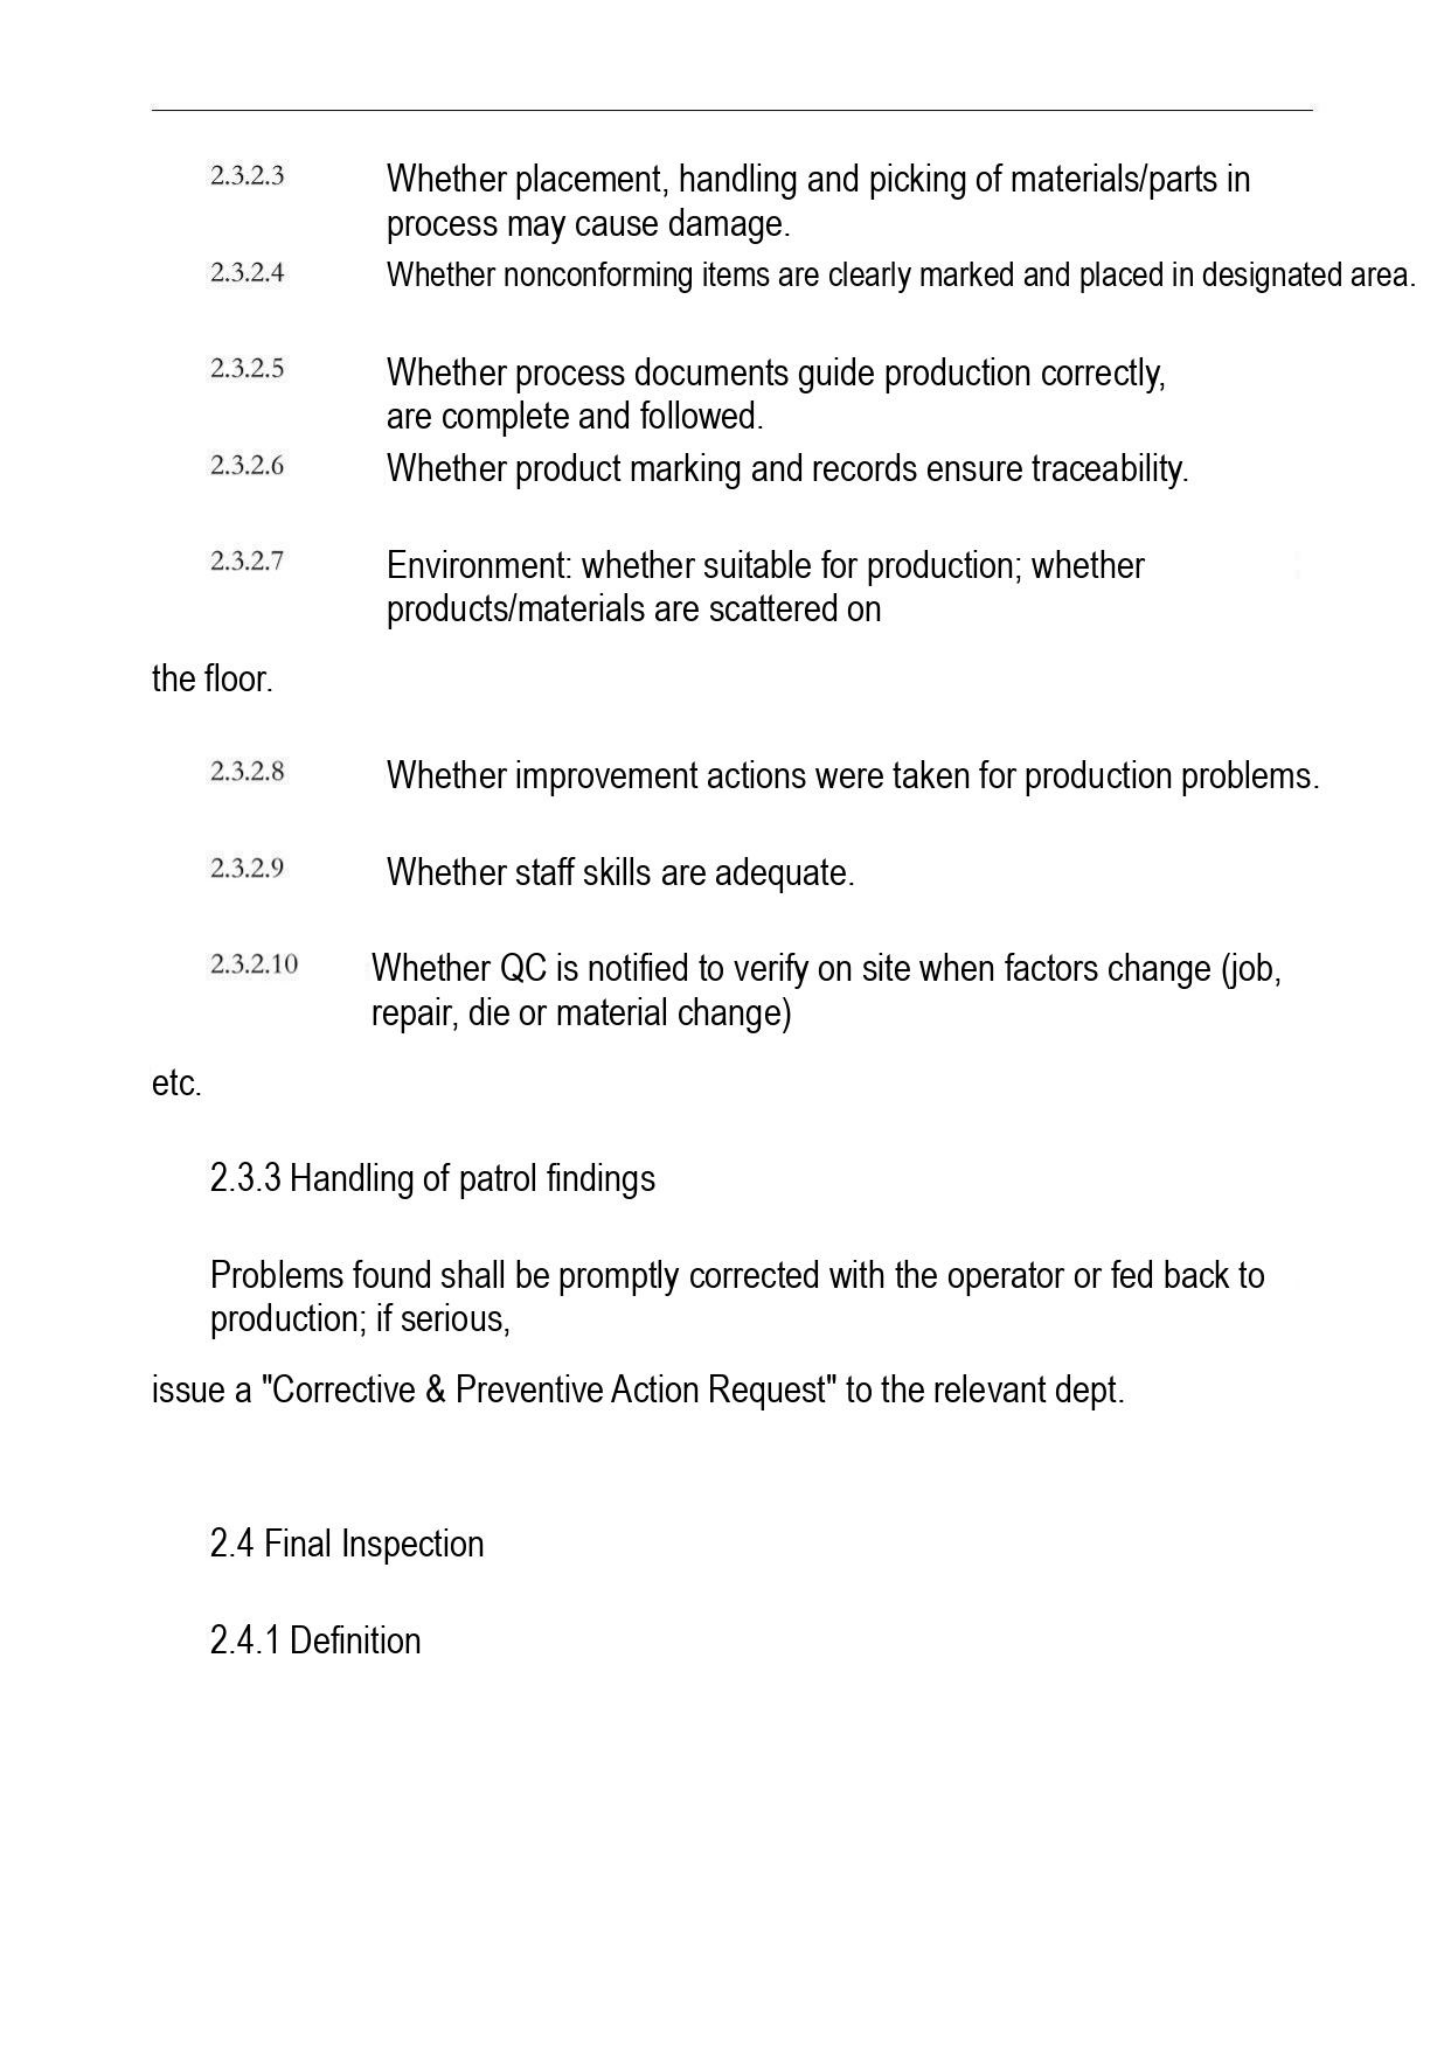2.3.2.3 Whether placement, handling and picking of materials/parts in process may cause damage.

2.3.2.4 Whether nonconforming items are clearly marked and placed in designated area.

2.3.2.5 Whether process documents guide production correctly, are complete and followed.

2.3.2.6 Whether product marking and records ensure traceability.

2.3.2.7 Environment: whether suitable for production; whether products/materials are scattered on

the floor.

2.3.2.8 Whether improvement actions were taken for production problems.

2.3.2.9 Whether staff skills are adequate.

2.3.2.10 Whether QC is notified to verify on site when factors change (job, repair, die or material change)

etc.

2.3.3 Handling of patrol findings

Problems found shall be promptly corrected with the operator or fed back to production; if serious,

issue a "Corrective & Preventive Action Request" to the relevant dept.

2.4 Final Inspection

2.4.1 Definition
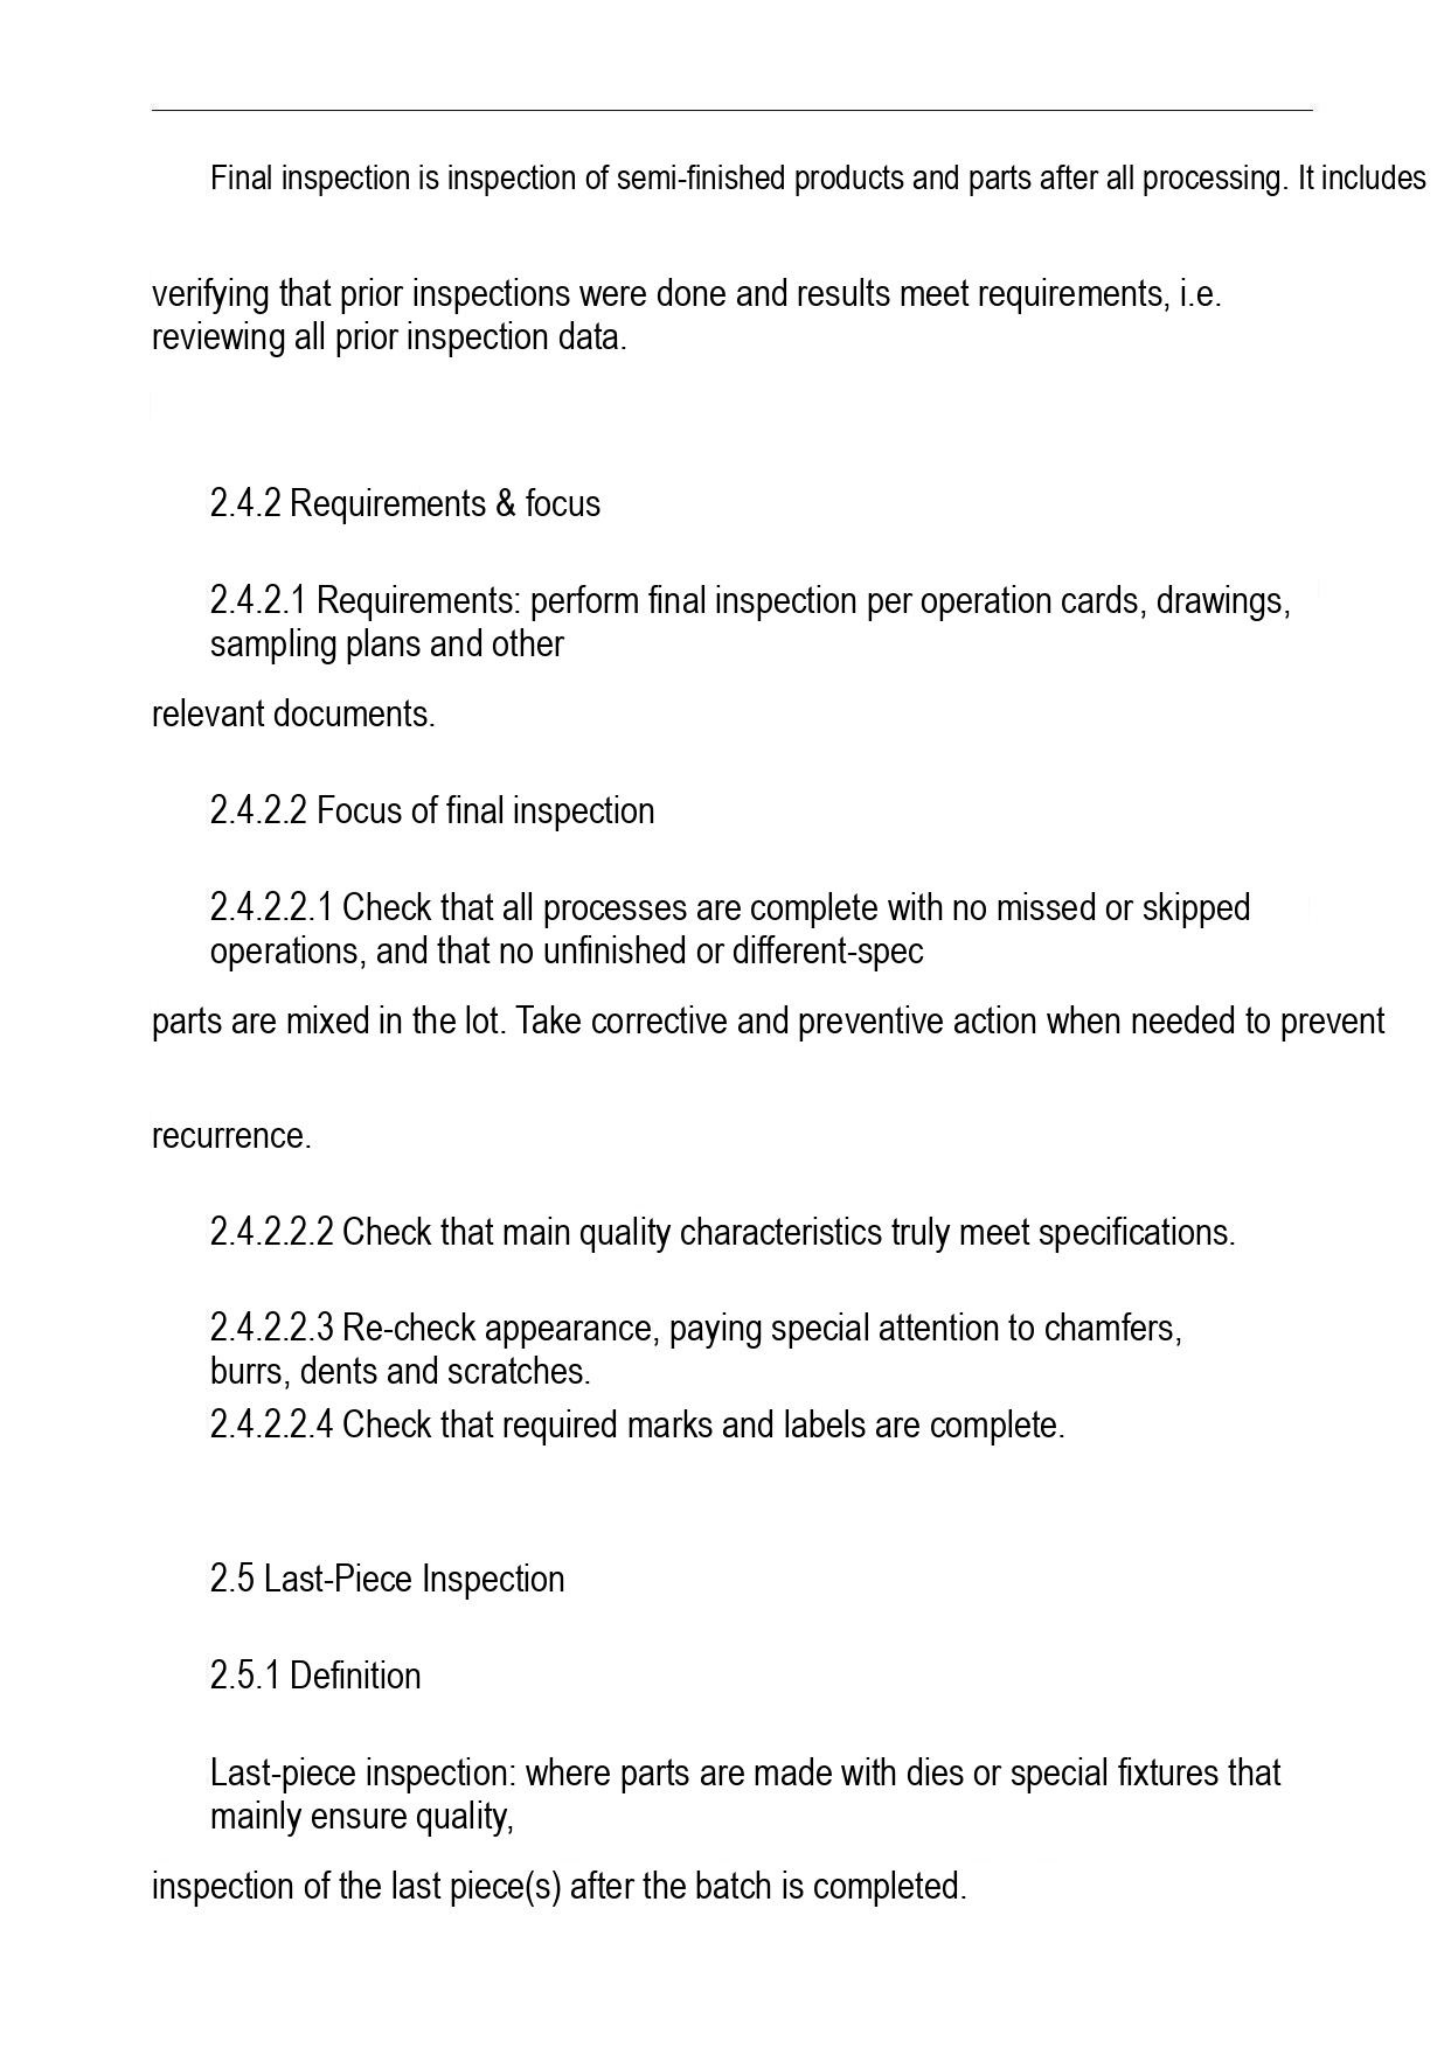Final inspection is inspection of semi-finished products and parts after all processing. It includes verifying that prior inspections were done and results meet requirements, i.e. reviewing all prior inspection data.

2.4.2 Requirements & focus

2.4.2.1 Requirements: perform final inspection per operation cards, drawings, sampling plans and other relevant documents.

2.4.2.2 Focus of final inspection

2.4.2.2.1 Check that all processes are complete with no missed or skipped operations, and that no unfinished or different-spec parts are mixed in the lot. Take corrective and preventive action when needed to prevent recurrence.

2.4.2.2.2 Check that main quality characteristics truly meet specifications.

2.4.2.2.3 Re-check appearance, paying special attention to chamfers, burrs, dents and scratches.

2.4.2.2.4 Check that required marks and labels are complete.

2.5 Last-Piece Inspection

2.5.1 Definition

Last-piece inspection: where parts are made with dies or special fixtures that mainly ensure quality, inspection of the last piece(s) after the batch is completed.
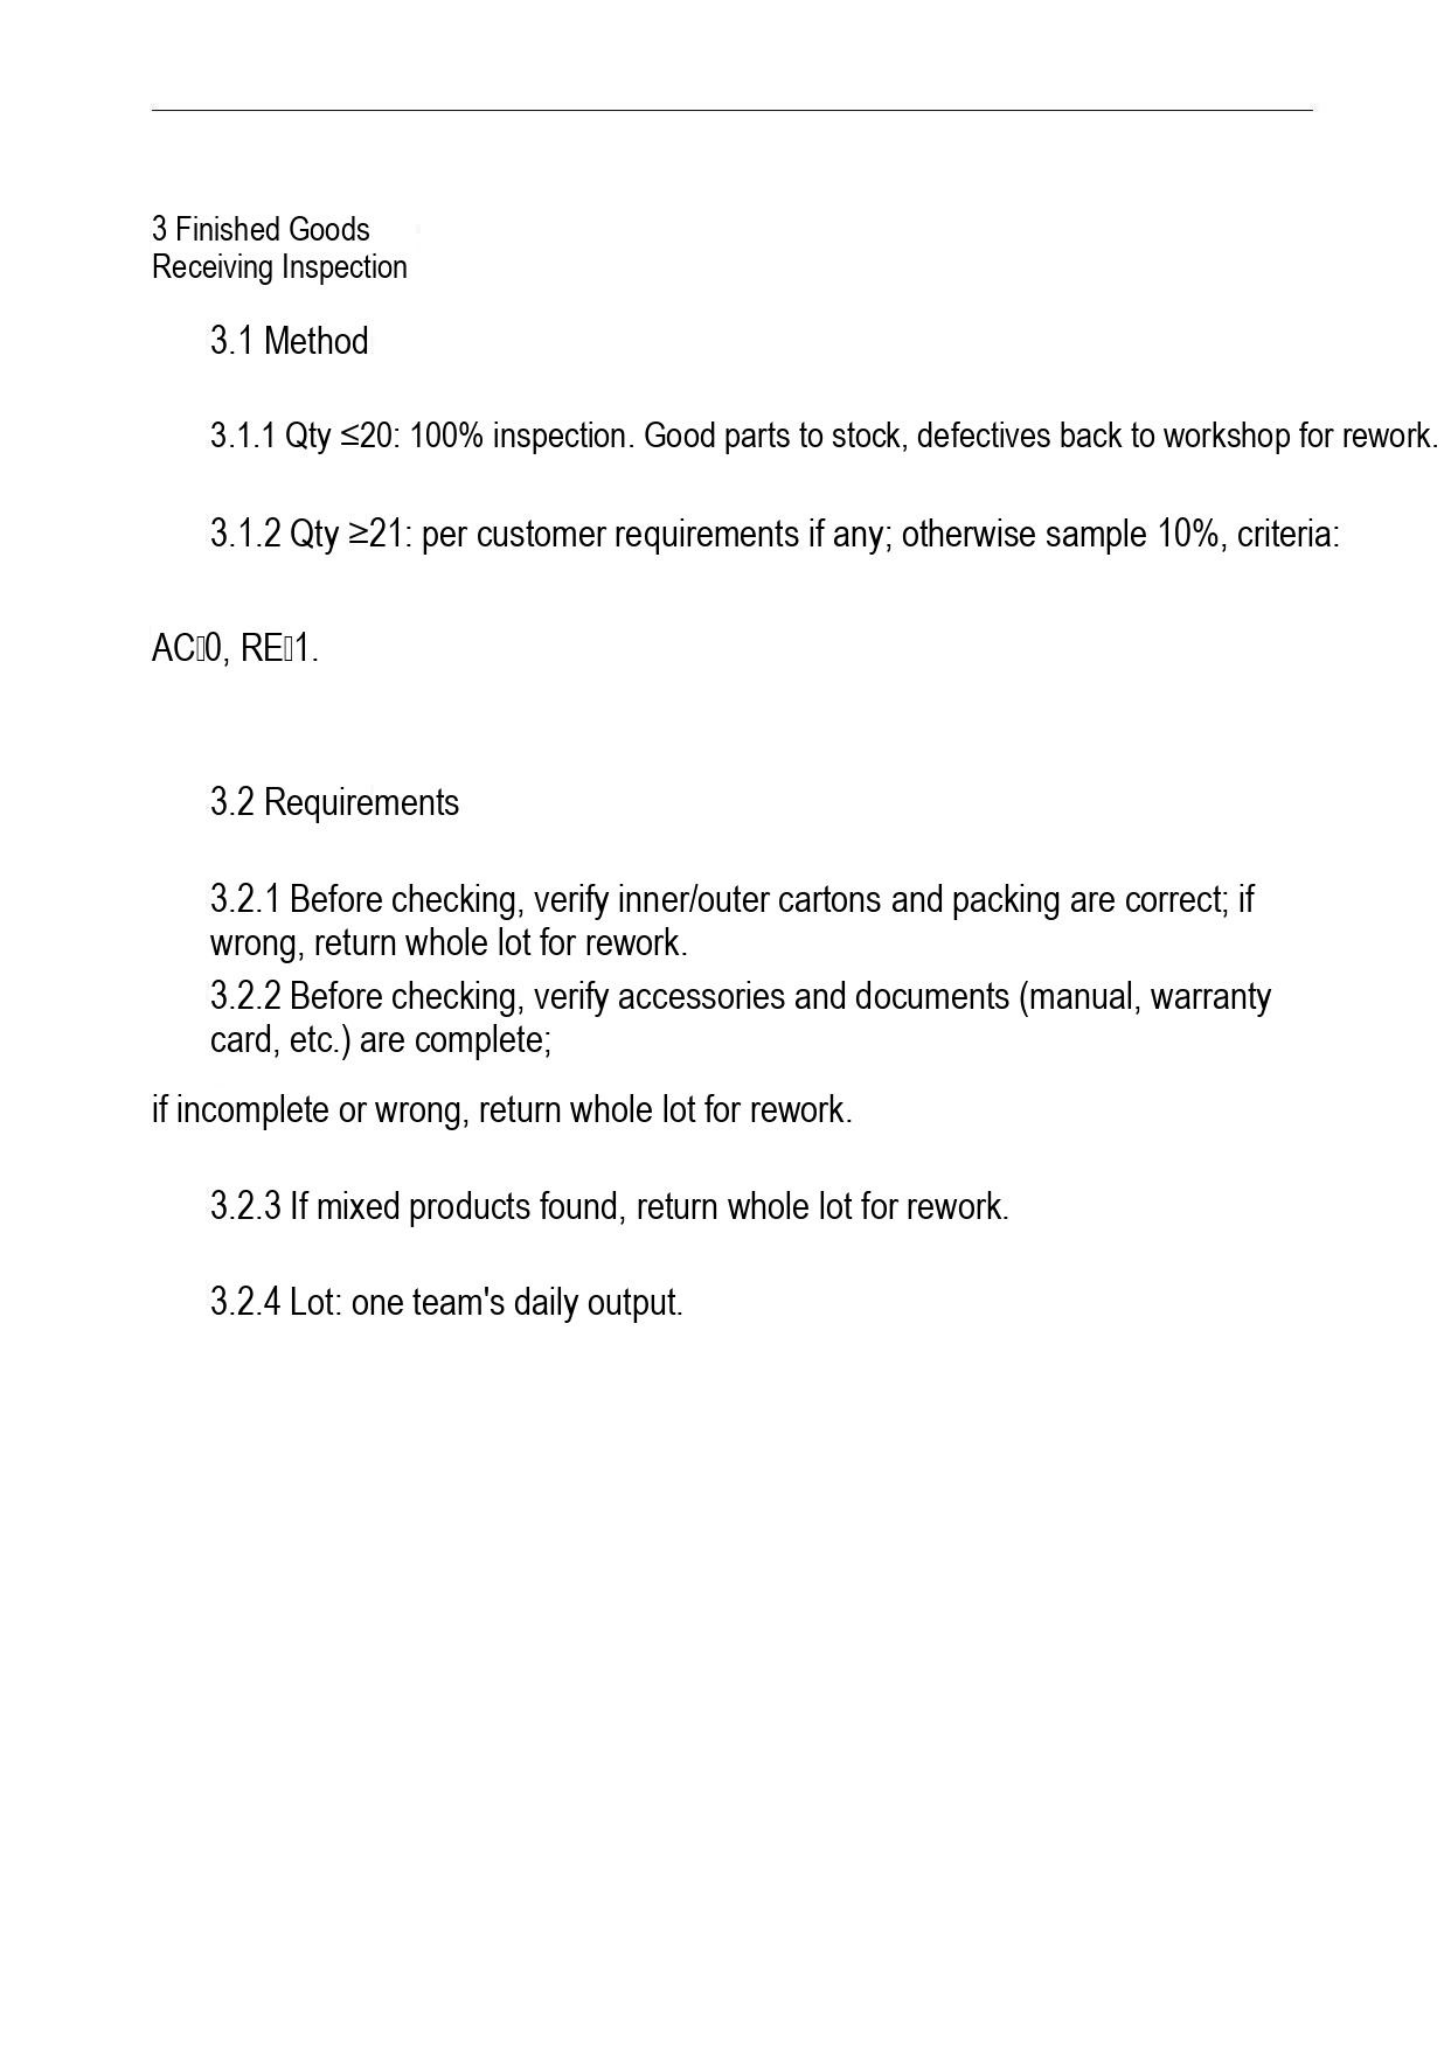3 Finished Goods
Receiving Inspection

3.1 Method

3.1.1 Qty ≤20: 100% inspection. Good parts to stock, defectives back to workshop for rework.

3.1.2 Qty ≥21: per customer requirements if any; otherwise sample 10%, criteria:

AC0, RE1.

3.2 Requirements

3.2.1 Before checking, verify inner/outer cartons and packing are correct; if wrong, return whole lot for rework.

3.2.2 Before checking, verify accessories and documents (manual, warranty card, etc.) are complete;

if incomplete or wrong, return whole lot for rework.

3.2.3 If mixed products found, return whole lot for rework.

3.2.4 Lot: one team's daily output.
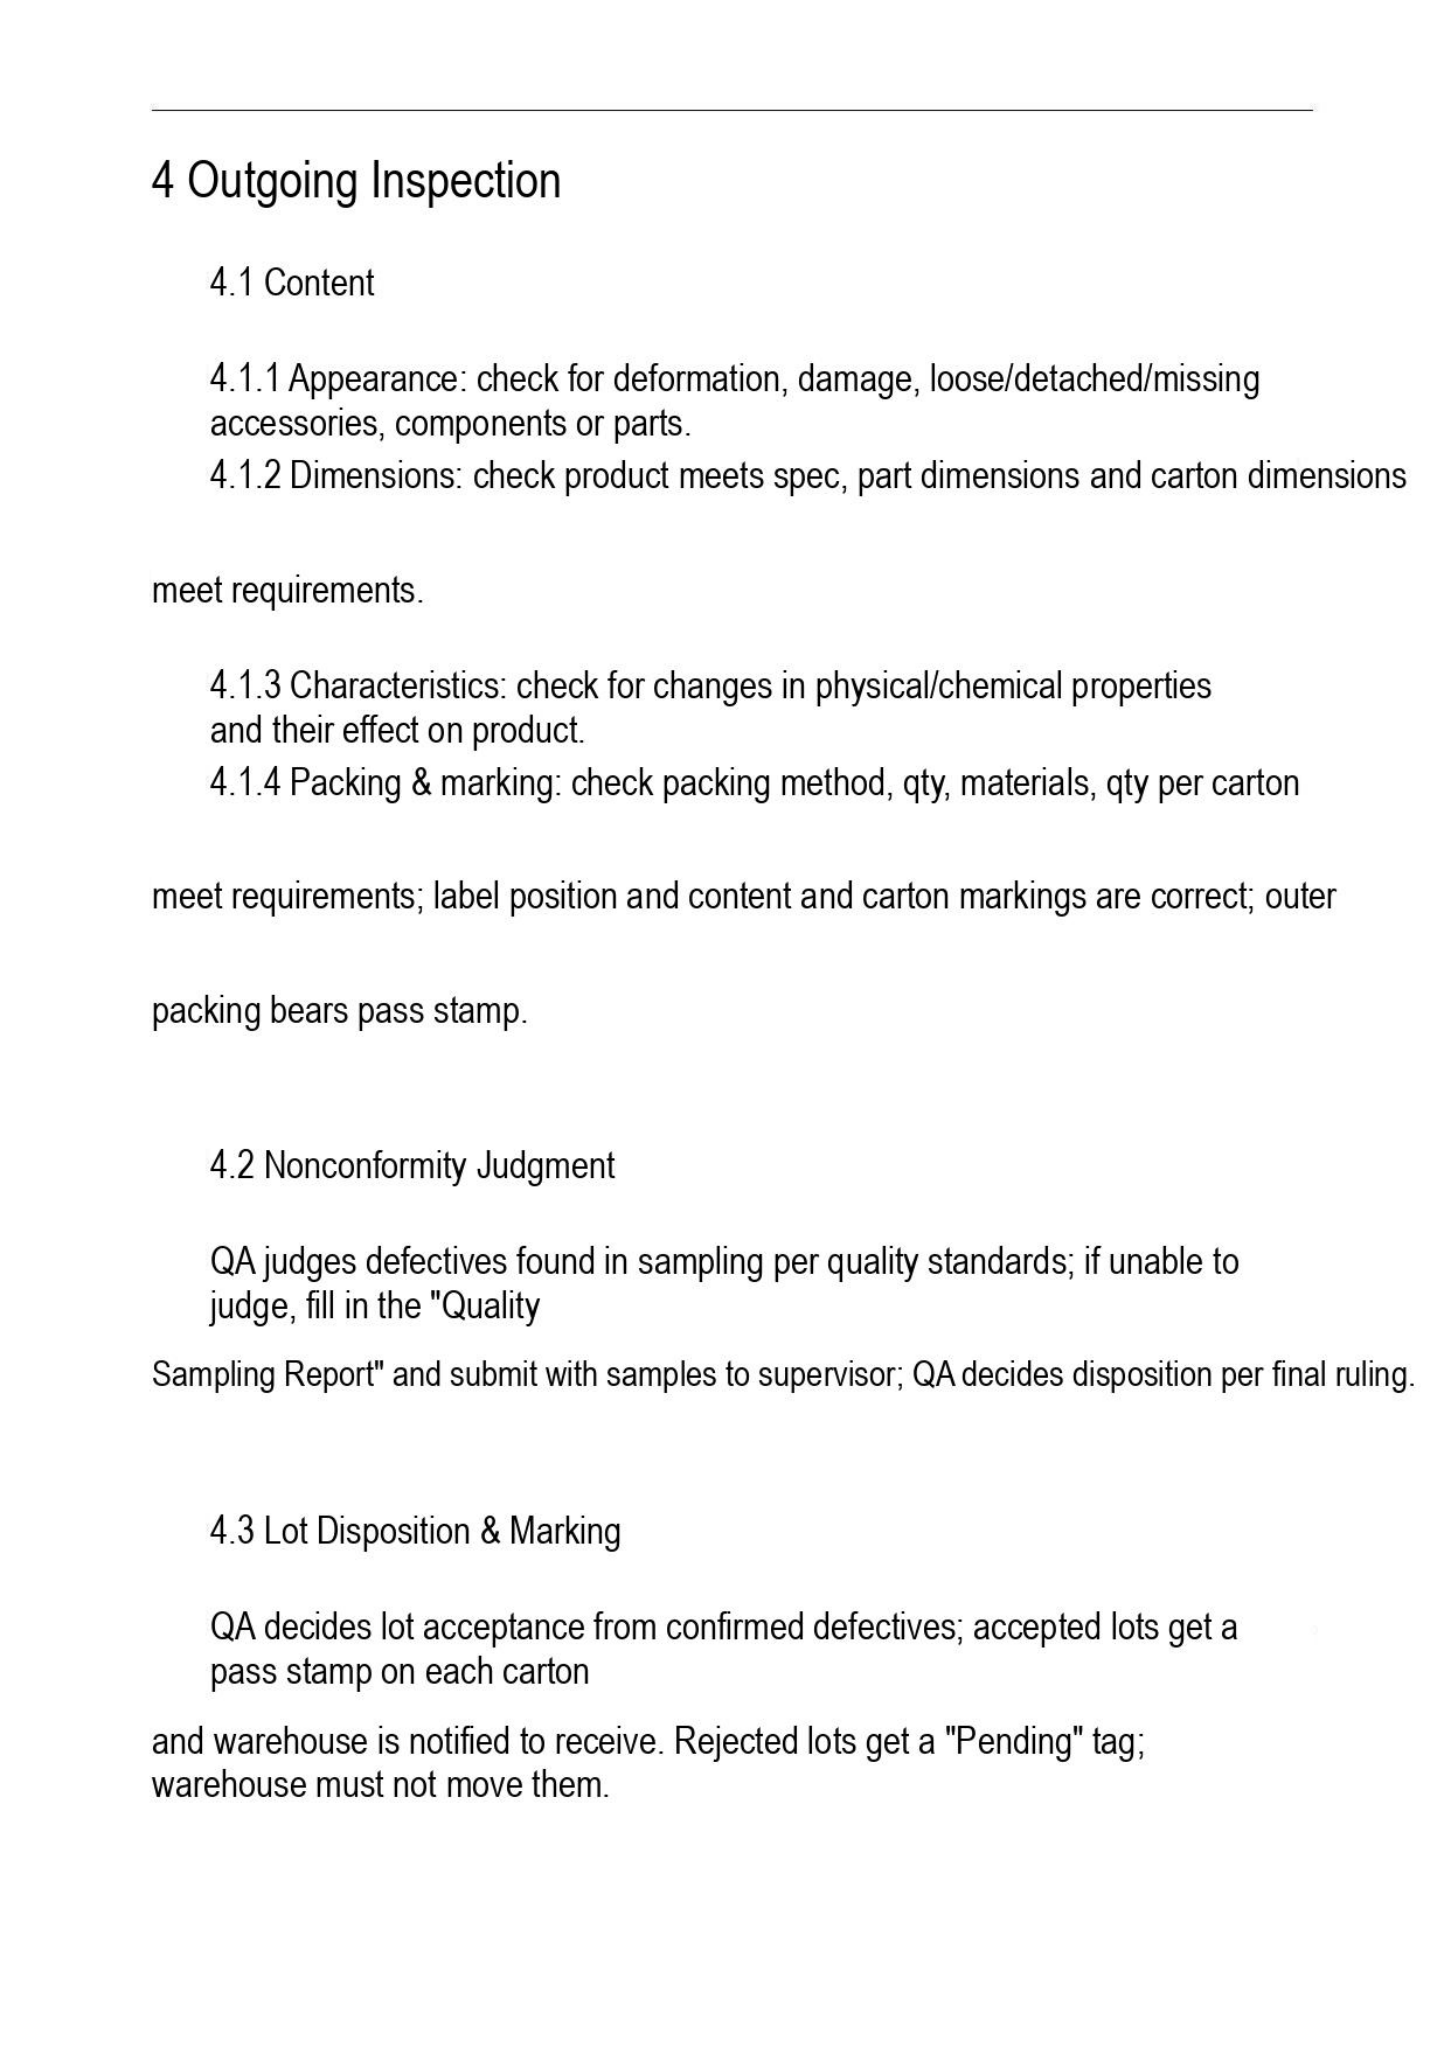4 Outgoing Inspection

4.1 Content

4.1.1 Appearance: check for deformation, damage, loose/detached/missing accessories, components or parts.
4.1.2 Dimensions: check product meets spec, part dimensions and carton dimensions

meet requirements.

4.1.3 Characteristics: check for changes in physical/chemical properties and their effect on product.
4.1.4 Packing & marking: check packing method, qty, materials, qty per carton

meet requirements; label position and content and carton markings are correct; outer

packing bears pass stamp.

4.2 Nonconformity Judgment

QA judges defectives found in sampling per quality standards; if unable to judge, fill in the "Quality

Sampling Report" and submit with samples to supervisor; QA decides disposition per final ruling.

4.3 Lot Disposition & Marking

QA decides lot acceptance from confirmed defectives; accepted lots get a pass stamp on each carton

and warehouse is notified to receive. Rejected lots get a "Pending" tag; warehouse must not move them.